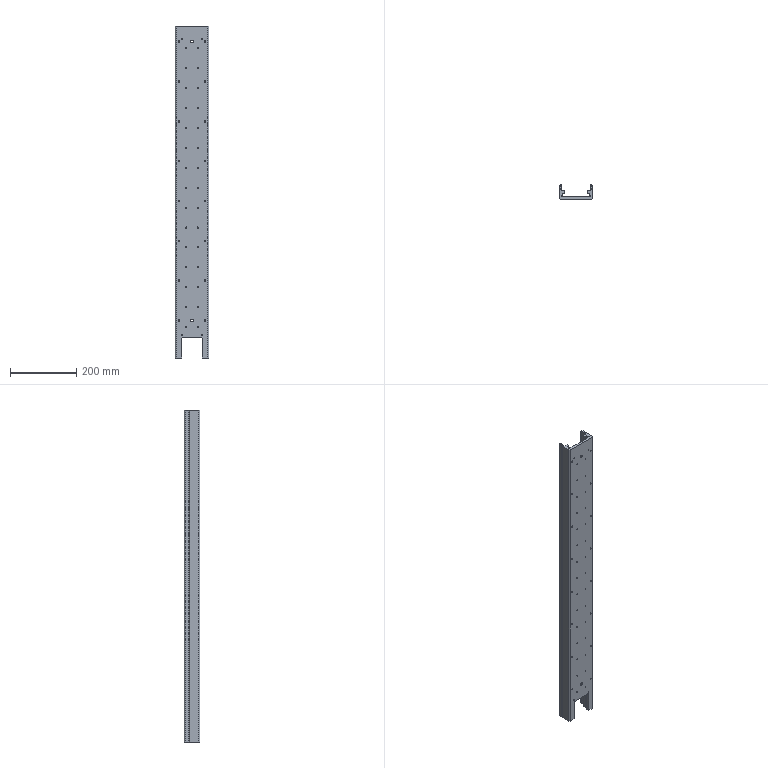Part | SolidWorks | features HoleWzd 6, ICE 6, MirrorPattern 4, Fillet 3, LPattern 3, Chamfer 1, Extrusion 1 | 1 solid | 277 faces | box 100 x 46 x 1000 mm | volume 1360190 mm3 | cylinder 197 | plane 64 | cone 16 | commonest cylinder face diameters 3.3 x96 7.99 x48 4.5 x32 3.2 x8 0.7 x4 8 x4